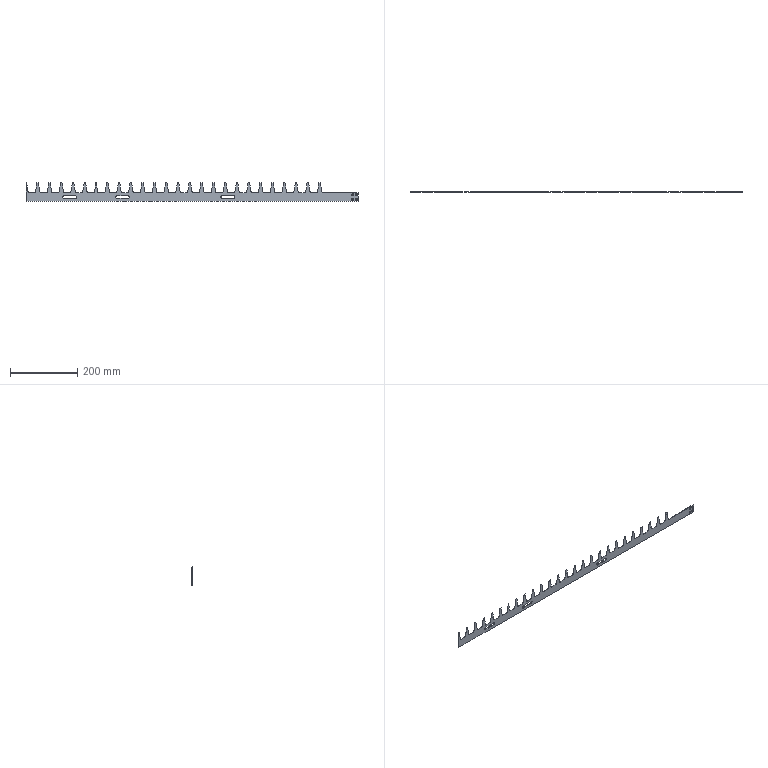Part | SolidWorks | features BaseBody 1, HoleWzd 1, ICE 1, MirrorSolid 1 | 1 solid | 193 faces | box 984.736 x 2.5 x 55 mm | volume 69770 mm3 | plane 117 | cone 62 | cylinder 14 | commonest cylinder face diameters 3.4 x8 8 x6